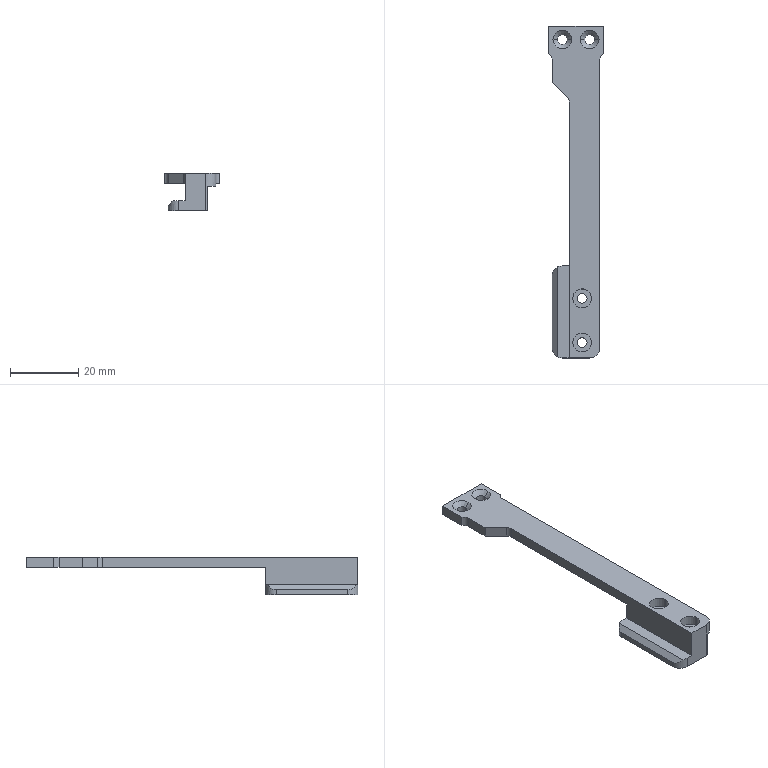CAM job | NX | 3-axis milling, drilling | part box 16 x 97.4 x 11 mm | stock box 23.6 x 101.4 x 15 mm
Tools:
number,name,description,diameter,corner_radius,flute_length,length,flutes
10,D2-6-D4-50-3T-ROUGH,D2-6-D4-50-3T-粗,2.0,0.0,6.0,7.0,2
5,D3-9-D4-50-3T-ROUGH,D3-9-D4-50-3T,3.0,0.0,9.0,10.0,3
6,D4-12-D4-50-3T-FINISH,D4-12-D4-50-3T,4.0,0.0,12.0,50.0,3
2,D8-25-D8-60-3T-ROUGH,D8-25-D8-60-3T-粗,8.0,0.0,25.0,60.0,2
1,D50面刀,D50面刀,50.0,0.0,30.0,30.0,4
4,钻头D2.9-39-67,钻刀D2.8-39-67,2.9,0.0,39.0,67.0,2
3,倒角D6-90度,倒角D6-90度,6.0,0.0,5.0,50.0,2
Operations:
program,operation,operation_type,tool,method,geometry_group,spindle_rpm,surface_speed,feed_per_tooth,feed_cut,feed_plunge,cut_length_mm,path_length_mm,cut_time_min,machine_time_min
A1,PLANAR_MILL,PlanarMilling,D50面刀,METHOD,WORKPIECE,4500.0,706.0,0.0556,1000.0,100.0,169.0,205.0,0.169,0.1726
A1,ADAPTIVE_MILLING,CavityMilling,D8-25-D8-60-3T-ROUGH,METHOD,WORKPIECE,6500.0,163.0,0.2308,3000.0,100.0,2270.658,2439.67,0.6025,0.6194
A1,ADAPTIVE_MILLING_COPY,CavityMilling,D8-25-D8-60-3T-ROUGH,METHOD,WORKPIECE,6500.0,163.0,0.2308,3000.0,100.0,457.881,507.581,0.0952,0.1002
A1,DRILLING,Operation,倒角D6-90度,METHOD,WORKPIECE,2500.0,47.0,0.04,200.0,0.0,11.7,79.742,0.0585,0.0653
A1,DRILLING_COPY,Operation,倒角D6-90度,METHOD,WORKPIECE,2500.0,47.0,0.04,200.0,0.0,11.5,74.544,0.0575,0.0638
A1,PLANAR_MILL_4,PlanarMilling,倒角D6-90度,METHOD,WORKPIECE,3000.0,56.0,0.1,600.0,100.0,39.196,96.196,0.0653,0.071
A1,PLANAR_MILL_3_COPY_1,PlanarMilling,倒角D6-90度,METHOD,WORKPIECE,3500.0,65.0,0.1429,1000.0,100.0,241.93,280.93,0.2419,0.2458
A1,DRILLING_COPY_1,Operation,钻头D2.9-39-67,METHOD,WORKPIECE,3000.0,27.0,0.0333,200.0,0.0,36.0,128.342,0.18,0.1892
A1,DRILLING_COPY_COPY,Operation,钻头D2.9-39-67,METHOD,WORKPIECE,3000.0,27.0,0.0333,200.0,0.0,18.0,87.544,0.09,0.097
A1,PLANAR_MILL_1,PlanarMilling,D3-9-D4-50-3T-ROUGH,METHOD,WORKPIECE,4500.0,42.0,0.0593,800.0,100.0,169.555,267.136,0.2119,0.2217
A1,PLANAR_MILL_1_COPY,PlanarMilling,D3-9-D4-50-3T-ROUGH,METHOD,WORKPIECE,4500.0,42.0,0.0444,600.0,100.0,33.991,130.591,0.0567,0.0663
A1,PLANAR_MILL_2,PlanarMilling,D3-9-D4-50-3T-ROUGH,METHOD,WORKPIECE,4500.0,42.0,0.0444,600.0,100.0,36.453,201.292,0.0608,0.0772
A1,PLANAR_MILL_3,PlanarMilling,D4-12-D4-50-3T-FINISH,METHOD,WORKPIECE,4500.0,56.0,0.0593,800.0,100.0,489.97,541.97,0.6125,0.6177
A1,PLANAR_MILL_3_COPY,PlanarMilling,D4-12-D4-50-3T-FINISH,METHOD,WORKPIECE,4500.0,56.0,0.0593,800.0,100.0,99.708,254.98,0.1246,0.1402
B1,ADAPTIVE_MILLING_1,CavityMilling,D8-25-D8-60-3T-ROUGH,METHOD,WORKPIECE_55,6500.0,163.0,0.2308,3000.0,100.0,6113.867,6317.809,1.566,1.586
B1,PLANAR_MILL_5_COPY,PlanarMilling,D4-12-D4-50-3T-FINISH,METHOD,WORKPIECE_55,6500.0,163.0,0.041,800.0,100.0,38.916,89.316,0.0486,0.0537
B1,PLANAR_MILL_5_COPY_1,PlanarMilling,D4-12-D4-50-3T-FINISH,METHOD,WORKPIECE_55,6500.0,163.0,0.041,800.0,100.0,33.991,85.991,0.0425,0.0477
B1,PLANAR_MILL_8,PlanarMilling,D50面刀,METHOD,B-G55,4500.0,706.0,0.0333,600.0,100.0,84.916,120.916,0.1415,0.1451
B1,PLANAR_MILL_10,PlanarMilling,D50面刀,METHOD,B-G55,4500.0,706.0,0.0333,600.0,100.0,175.8,368.902,0.293,0.3123
B1,DRILLING_1,Operation,倒角D6-90度,METHOD,WORKPIECE_55,3000.0,56.0,0.0333,200.0,0.0,9.1,74.542,0.0455,0.052
B1,DRILLING_1_COPY,Operation,倒角D6-90度,METHOD,WORKPIECE_55,3000.0,56.0,0.0333,200.0,0.0,9.1,85.744,0.0455,0.0532
B1,PLANAR_MILL_6,PlanarMilling,倒角D6-90度,METHOD,WORKPIECE_55,3500.0,65.0,0.1429,1000.0,100.0,90.991,129.991,0.091,0.0949
B1,PLANAR_MILL_6_COPY,PlanarMilling,倒角D6-90度,METHOD,WORKPIECE_55,3500.0,65.0,0.1429,1000.0,100.0,28.142,81.542,0.0281,0.0335
B1,PLANAR_MILL_6_COPY_1,PlanarMilling,倒角D6-90度,METHOD,WORKPIECE_55,3500.0,65.0,0.1429,1000.0,100.0,164.691,219.691,0.1647,0.1702
B10,PLANAR_MILL_9,PlanarMilling,D4-12-D4-50-3T-FINISH,METHOD,B-G55,6500.0,163.0,0.041,800.0,100.0,348.078,398.038,0.4351,0.4401
B10,PLANAR_MILL_9_COPY,PlanarMilling,D4-12-D4-50-3T-FINISH,METHOD,B-G55,6500.0,163.0,0.041,800.0,100.0,348.078,398.078,0.4351,0.4401
B10,PLANAR_MILL_5,PlanarMilling,D4-12-D4-50-3T-FINISH,METHOD,WORKPIECE_55,6500.0,163.0,0.041,800.0,100.0,33.991,85.945,0.0425,0.0477
工装1,PLANAR_MILL_7,PlanarMilling,D2-6-D4-50-3T-ROUGH,METHOD,GZ1,6500.0,40.0,0.0923,1200.0,100.0,6275.655,6745.483,5.23,5.277
工装1,PLANAR_MILL_7_COPY,PlanarMilling,D2-6-D4-50-3T-ROUGH,METHOD,GZ1,6500.0,40.0,0.0615,800.0,100.0,882.495,947.095,1.103,1.11
工装1,PLANAR_MILL_7_COPY_COPY,PlanarMilling,D2-6-D4-50-3T-ROUGH,METHOD,GZ1,6500.0,40.0,0.0615,800.0,100.0,253.259,314.859,0.3166,0.3227